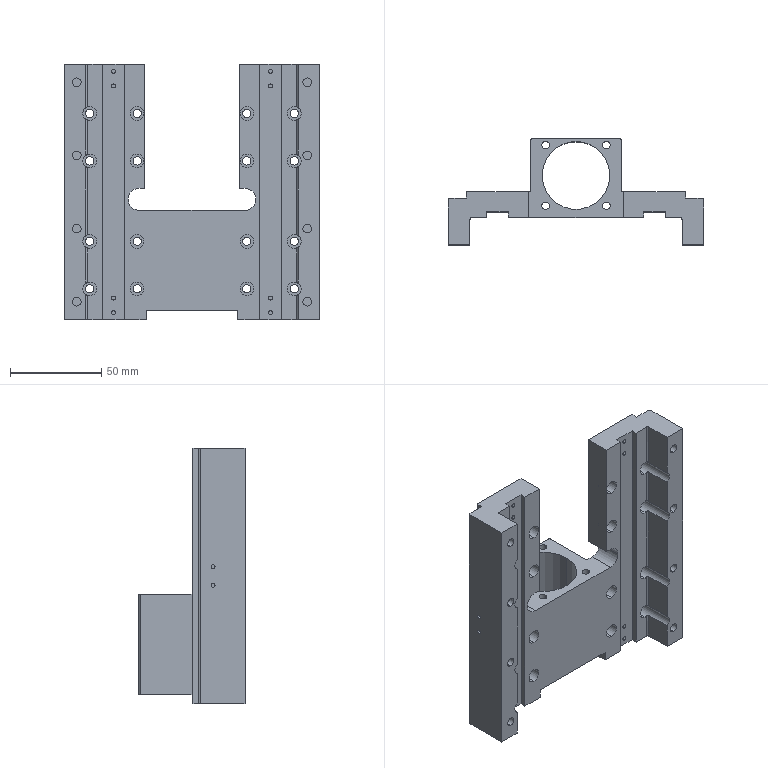Part | STEP file | SM140A-20-1140D-Slide plate 140-1000-2 | 1 solid | 213 faces | box 140 x 58 x 140 mm | volume 247713 mm3 | cylinder 133 | plane 80 | commonest cylinder face diameters 4.5 x32 7.5 x32 2.2 x24 2 x16 4.8 x16 4.2 x8